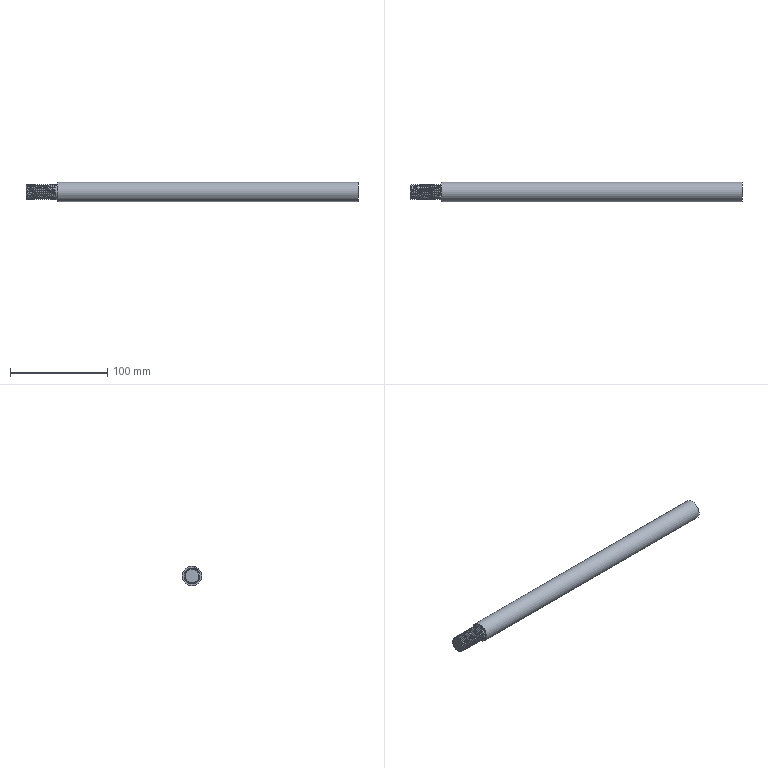Part | STEP file | Tube feed_id394_x_t | 1 solid | 11 faces | box 342 x 20 x 20 mm | volume 102696 mm3 | plane 4 | cylinder 3 | spline 3 | cone 1 | commonest cylinder face diameters 14 x1 16 x1 20 x1